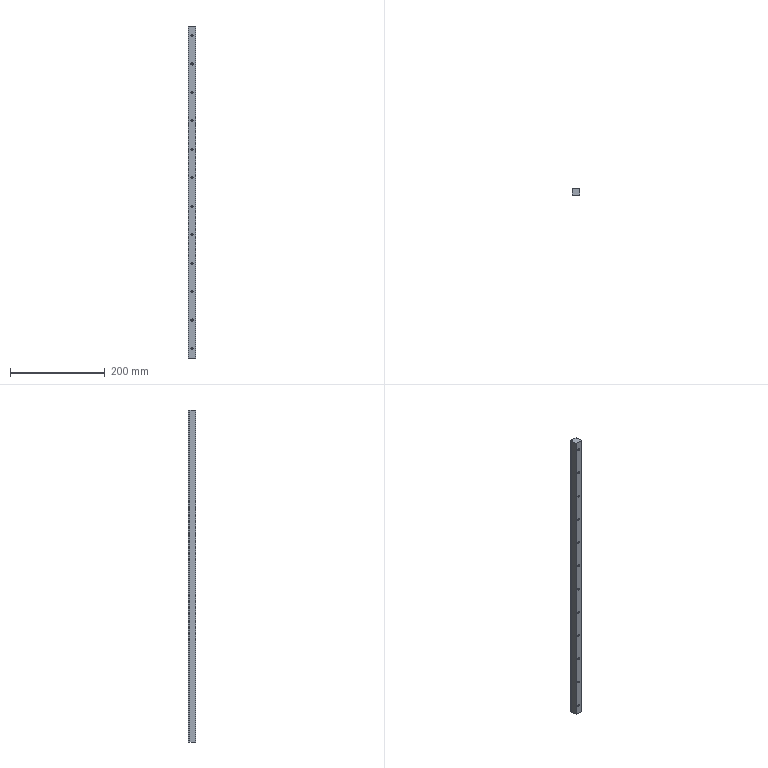Part | STEP file | 1 solid | 46 faces | box 15 x 15 x 700 mm | volume 150376 mm3 | cylinder 26 | plane 20 | commonest cylinder face diameters 4.5 x12 8 x12 2 x2